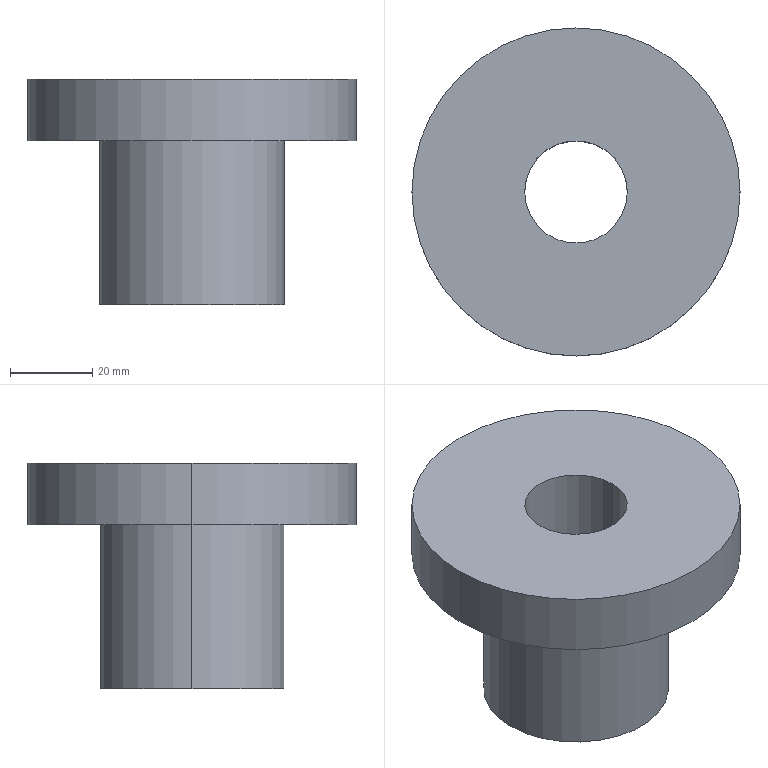Part | SolidWorks | features Cut 1, Extrusion 1, ICE 1 | 1 solid | 9 faces | box 80 x 80 x 55 mm | volume 112017 mm3 | cylinder 6 | plane 3 | commonest cylinder face diameters 25 x2 45 x2 80 x2
STEP:
#1=CARTESIAN_POINT('',(-12.5,0.,55.));
#2=VERTEX_POINT('',#1);
#3=CARTESIAN_POINT('',(12.5,0.,55.));
#4=VERTEX_POINT('',#3);
#5=CARTESIAN_POINT('',(0.,0.,55.));
#6=DIRECTION('',(0.,0.,1.));
#7=DIRECTION('',(1.,0.,0.));
#8=AXIS2_PLACEMENT_3D('',#5,#6,#7);
#9=CIRCLE('',#8,12.5);
#10=EDGE_CURVE('',#2,#4,#9,.T.);
#11=ORIENTED_EDGE('',*,*,#10,.T.);
#12=CARTESIAN_POINT('',(12.5,0.,0.));
#13=VERTEX_POINT('',#12);
#14=CARTESIAN_POINT('',(12.5,0.,97.));
#15=DIRECTION('',(0.,0.,-1.));
#16=VECTOR('',#15,1000.);
#17=LINE('',#14,#16);
#18=EDGE_CURVE('',#4,#13,#17,.T.);
#19=ORIENTED_EDGE('',*,*,#18,.T.);
#20=CARTESIAN_POINT('',(-12.5,0.,0.));
#21=VERTEX_POINT('',#20);
#22=CARTESIAN_POINT('',(0.,0.,0.));
#23=DIRECTION('',(0.,0.,-1.));
#24=DIRECTION('',(-1.,0.,0.));
#25=AXIS2_PLACEMENT_3D('',#22,#23,#24);
#26=CIRCLE('',#25,12.5);
#27=EDGE_CURVE('',#13,#21,#26,.T.);
#28=ORIENTED_EDGE('',*,*,#27,.T.);
#29=CARTESIAN_POINT('',(-12.5,0.,97.));
#30=DIRECTION('',(0.,0.,-1.));
#31=VECTOR('',#30,1000.);
#32=LINE('',#29,#31);
#33=EDGE_CURVE('',#2,#21,#32,.T.);
#34=ORIENTED_EDGE('',*,*,#33,.F.);
#35=EDGE_LOOP('',(#11,#19,#28,#34));
#36=FACE_OUTER_BOUND('',#35,.T.);
#37=CARTESIAN_POINT('',(0.,0.,97.));
#38=DIRECTION('',(0.,0.,-1.));
#39=DIRECTION('',(-1.,0.,0.));
#40=AXIS2_PLACEMENT_3D('',#37,#38,#39);
#41=CYLINDRICAL_SURFACE('',#40,12.5);
#42=ADVANCED_FACE('',(#36),#41,.F.);
#43=CARTESIAN_POINT('',(40.,0.,55.));
#44=VERTEX_POINT('',#43);
#45=CARTESIAN_POINT('',(-40.,0.,55.));
#46=VERTEX_POINT('',#45);
#47=CARTESIAN_POINT('',(0.,0.,55.));
#48=DIRECTION('',(0.,0.,1.));
#49=DIRECTION('',(1.,0.,0.));
#50=AXIS2_PLACEMENT_3D('',#47,#48,#49);
#51=CIRCLE('',#50,40.);
#52=EDGE_CURVE('',#44,#46,#51,.T.);
#53=ORIENTED_EDGE('',*,*,#52,.F.);
#54=CARTESIAN_POINT('',(40.,0.,40.));
#55=VERTEX_POINT('',#54);
#56=CARTESIAN_POINT('',(40.,0.,55.));
#57=DIRECTION('',(0.,0.,-1.));
#58=VECTOR('',#57,1000.);
#59=LINE('',#56,#58);
#60=EDGE_CURVE('',#44,#55,#59,.T.);
#61=ORIENTED_EDGE('',*,*,#60,.T.);
#62=CARTESIAN_POINT('',(-40.,0.,40.));
#63=VERTEX_POINT('',#62);
#64=CARTESIAN_POINT('',(0.,0.,40.));
#65=DIRECTION('',(0.,0.,1.));
#66=DIRECTION('',(1.,0.,0.));
#67=AXIS2_PLACEMENT_3D('',#64,#65,#66);
#68=CIRCLE('',#67,40.);
#69=EDGE_CURVE('',#55,#63,#68,.T.);
#70=ORIENTED_EDGE('',*,*,#69,.T.);
#71=CARTESIAN_POINT('',(-40.,0.,55.));
#72=DIRECTION('',(0.,0.,-1.));
#73=VECTOR('',#72,1000.);
#74=LINE('',#71,#73);
#75=EDGE_CURVE('',#46,#63,#74,.T.);
#76=ORIENTED_EDGE('',*,*,#75,.F.);
#77=EDGE_LOOP('',(#53,#61,#70,#76));
#78=FACE_OUTER_BOUND('',#77,.T.);
#79=CARTESIAN_POINT('',(0.,0.,55.));
#80=DIRECTION('',(0.,0.,-1.));
#81=DIRECTION('',(-1.,0.,0.));
#82=AXIS2_PLACEMENT_3D('',#79,#80,#81);
#83=CYLINDRICAL_SURFACE('',#82,40.);
#84=ADVANCED_FACE('',(#78),#83,.T.);
#85=CARTESIAN_POINT('',(22.5,0.,40.));
#86=VERTEX_POINT('',#85);
#87=CARTESIAN_POINT('',(-22.5,0.,40.));
#88=VERTEX_POINT('',#87);
#89=CARTESIAN_POINT('',(0.,0.,40.));
#90=DIRECTION('',(0.,0.,1.));
#91=DIRECTION('',(1.,0.,0.));
#92=AXIS2_PLACEMENT_3D('',#89,#90,#91);
#93=CIRCLE('',#92,22.5);
#94=EDGE_CURVE('',#86,#88,#93,.T.);
#95=ORIENTED_EDGE('',*,*,#94,.F.);
#96=CARTESIAN_POINT('',(22.5,0.,0.));
#97=VERTEX_POINT('',#96);
#98=CARTESIAN_POINT('',(22.5,0.,40.));
#99=DIRECTION('',(0.,0.,-1.));
#100=VECTOR('',#99,1000.);
#101=LINE('',#98,#100);
#102=EDGE_CURVE('',#86,#97,#101,.T.);
#103=ORIENTED_EDGE('',*,*,#102,.T.);
#104=CARTESIAN_POINT('',(-22.5,0.,0.));
#105=VERTEX_POINT('',#104);
#106=CARTESIAN_POINT('',(0.,0.,0.));
#107=DIRECTION('',(0.,0.,1.));
#108=DIRECTION('',(1.,0.,0.));
#109=AXIS2_PLACEMENT_3D('',#106,#107,#108);
#110=CIRCLE('',#109,22.5);
#111=EDGE_CURVE('',#97,#105,#110,.T.);
#112=ORIENTED_EDGE('',*,*,#111,.T.);
#113=CARTESIAN_POINT('',(-22.5,0.,40.));
#114=DIRECTION('',(0.,0.,-1.));
#115=VECTOR('',#114,1000.);
#116=LINE('',#113,#115);
#117=EDGE_CURVE('',#88,#105,#116,.T.);
#118=ORIENTED_EDGE('',*,*,#117,.F.);
#119=EDGE_LOOP('',(#95,#103,#112,#118));
#120=FACE_OUTER_BOUND('',#119,.T.);
#121=CARTESIAN_POINT('',(0.,0.,40.));
#122=DIRECTION('',(0.,0.,-1.));
#123=DIRECTION('',(-1.,0.,0.));
#124=AXIS2_PLACEMENT_3D('',#121,#122,#123);
#125=CYLINDRICAL_SURFACE('',#124,22.5);
#126=ADVANCED_FACE('',(#120),#125,.T.);
#127=ORIENTED_EDGE('',*,*,#102,.F.);
#128=CARTESIAN_POINT('',(0.,0.,40.));
#129=DIRECTION('',(0.,0.,1.));
#130=DIRECTION('',(1.,0.,0.));
#131=AXIS2_PLACEMENT_3D('',#128,#129,#130);
#132=CIRCLE('',#131,22.5);
#133=EDGE_CURVE('',#88,#86,#132,.T.);
#134=ORIENTED_EDGE('',*,*,#133,.F.);
#135=ORIENTED_EDGE('',*,*,#117,.T.);
#136=CARTESIAN_POINT('',(0.,0.,0.));
#137=DIRECTION('',(0.,0.,1.));
#138=DIRECTION('',(1.,0.,0.));
#139=AXIS2_PLACEMENT_3D('',#136,#137,#138);
#140=CIRCLE('',#139,22.5);
#141=EDGE_CURVE('',#105,#97,#140,.T.);
#142=ORIENTED_EDGE('',*,*,#141,.T.);
#143=EDGE_LOOP('',(#127,#134,#135,#142));
#144=FACE_OUTER_BOUND('',#143,.T.);
#145=CARTESIAN_POINT('',(0.,0.,40.));
#146=DIRECTION('',(0.,0.,-1.));
#147=DIRECTION('',(-1.,0.,0.));
#148=AXIS2_PLACEMENT_3D('',#145,#146,#147);
#149=CYLINDRICAL_SURFACE('',#148,22.5);
#150=ADVANCED_FACE('',(#144),#149,.T.);
#151=CARTESIAN_POINT('',(0.,0.,0.));
#152=DIRECTION('',(0.,0.,-1.));
#153=DIRECTION('',(-1.,0.,0.));
#154=AXIS2_PLACEMENT_3D('',#151,#152,#153);
#155=CIRCLE('',#154,12.5);
#156=EDGE_CURVE('',#21,#13,#155,.T.);
#157=ORIENTED_EDGE('',*,*,#156,.F.);
#158=ORIENTED_EDGE('',*,*,#27,.F.);
#159=EDGE_LOOP('',(#157,#158));
#160=FACE_BOUND('',#159,.T.);
#161=ORIENTED_EDGE('',*,*,#141,.F.);
#162=ORIENTED_EDGE('',*,*,#111,.F.);
#163=EDGE_LOOP('',(#161,#162));
#164=FACE_OUTER_BOUND('',#163,.T.);
#165=CARTESIAN_POINT('',(0.,0.,0.));
#166=DIRECTION('',(0.,0.,1.));
#167=DIRECTION('',(1.,0.,0.));
#168=AXIS2_PLACEMENT_3D('',#165,#166,#167);
#169=PLANE('',#168);
#170=ADVANCED_FACE('',(#160,#164),#169,.F.);
#171=ORIENTED_EDGE('',*,*,#60,.F.);
#172=CARTESIAN_POINT('',(0.,0.,55.));
#173=DIRECTION('',(0.,0.,1.));
#174=DIRECTION('',(1.,0.,0.));
#175=AXIS2_PLACEMENT_3D('',#172,#173,#174);
#176=CIRCLE('',#175,40.);
#177=EDGE_CURVE('',#46,#44,#176,.T.);
#178=ORIENTED_EDGE('',*,*,#177,.F.);
#179=ORIENTED_EDGE('',*,*,#75,.T.);
#180=CARTESIAN_POINT('',(0.,0.,40.));
#181=DIRECTION('',(0.,0.,1.));
#182=DIRECTION('',(1.,0.,0.));
#183=AXIS2_PLACEMENT_3D('',#180,#181,#182);
#184=CIRCLE('',#183,40.);
#185=EDGE_CURVE('',#63,#55,#184,.T.);
#186=ORIENTED_EDGE('',*,*,#185,.T.);
#187=EDGE_LOOP('',(#171,#178,#179,#186));
#188=FACE_OUTER_BOUND('',#187,.T.);
#189=CARTESIAN_POINT('',(0.,0.,55.));
#190=DIRECTION('',(0.,0.,-1.));
#191=DIRECTION('',(-1.,0.,0.));
#192=AXIS2_PLACEMENT_3D('',#189,#190,#191);
#193=CYLINDRICAL_SURFACE('',#192,40.);
#194=ADVANCED_FACE('',(#188),#193,.T.);
#195=ORIENTED_EDGE('',*,*,#10,.F.);
#196=CARTESIAN_POINT('',(0.,0.,55.));
#197=DIRECTION('',(0.,0.,1.));
#198=DIRECTION('',(1.,0.,0.));
#199=AXIS2_PLACEMENT_3D('',#196,#197,#198);
#200=CIRCLE('',#199,12.5);
#201=EDGE_CURVE('',#4,#2,#200,.T.);
#202=ORIENTED_EDGE('',*,*,#201,.F.);
#203=EDGE_LOOP('',(#195,#202));
#204=FACE_BOUND('',#203,.T.);
#205=ORIENTED_EDGE('',*,*,#177,.T.);
#206=ORIENTED_EDGE('',*,*,#52,.T.);
#207=EDGE_LOOP('',(#205,#206));
#208=FACE_OUTER_BOUND('',#207,.T.);
#209=CARTESIAN_POINT('',(0.,0.,55.));
#210=DIRECTION('',(0.,0.,1.));
#211=DIRECTION('',(1.,0.,0.));
#212=AXIS2_PLACEMENT_3D('',#209,#210,#211);
#213=PLANE('',#212);
#214=ADVANCED_FACE('',(#204,#208),#213,.T.);
#215=ORIENTED_EDGE('',*,*,#133,.T.);
#216=ORIENTED_EDGE('',*,*,#94,.T.);
#217=EDGE_LOOP('',(#215,#216));
#218=FACE_BOUND('',#217,.T.);
#219=ORIENTED_EDGE('',*,*,#185,.F.);
#220=ORIENTED_EDGE('',*,*,#69,.F.);
#221=EDGE_LOOP('',(#219,#220));
#222=FACE_OUTER_BOUND('',#221,.T.);
#223=CARTESIAN_POINT('',(0.,0.,40.));
#224=DIRECTION('',(0.,0.,1.));
#225=DIRECTION('',(1.,0.,0.));
#226=AXIS2_PLACEMENT_3D('',#223,#224,#225);
#227=PLANE('',#226);
#228=ADVANCED_FACE('',(#218,#222),#227,.F.);
#229=ORIENTED_EDGE('',*,*,#18,.F.);
#230=ORIENTED_EDGE('',*,*,#201,.T.);
#231=ORIENTED_EDGE('',*,*,#33,.T.);
#232=ORIENTED_EDGE('',*,*,#156,.T.);
#233=EDGE_LOOP('',(#229,#230,#231,#232));
#234=FACE_OUTER_BOUND('',#233,.T.);
#235=CARTESIAN_POINT('',(0.,0.,97.));
#236=DIRECTION('',(0.,0.,-1.));
#237=DIRECTION('',(-1.,0.,0.));
#238=AXIS2_PLACEMENT_3D('',#235,#236,#237);
#239=CYLINDRICAL_SURFACE('',#238,12.5);
#240=ADVANCED_FACE('',(#234),#239,.F.);
#241=CLOSED_SHELL('',(#42,#84,#126,#150,#170,#194,#214,#228,#240));
#242=MANIFOLD_SOLID_BREP('',#241);
#243=CARTESIAN_POINT('',(0.,0.,0.));
#244=DIRECTION('',(0.,0.,1.));
#245=DIRECTION('',(1.,0.,0.));
#246=AXIS2_PLACEMENT_3D('',#243,#244,#245);
#247=(LENGTH_UNIT()NAMED_UNIT(*)SI_UNIT(.MILLI.,.METRE.));
#248=UNCERTAINTY_MEASURE_WITH_UNIT(LENGTH_MEASURE(0.00001),#247,'','');
#249=(NAMED_UNIT(*)PLANE_ANGLE_UNIT()SI_UNIT($,.RADIAN.));
#250=(NAMED_UNIT(*)SI_UNIT($,.STERADIAN.)SOLID_ANGLE_UNIT());
#251=(GEOMETRIC_REPRESENTATION_CONTEXT(3)GLOBAL_UNCERTAINTY_ASSIGNED_CONTEXT((#248))GLOBAL_UNIT_ASSIGNED_CONTEXT((#247,#249,#250))REPRESENTATION_CONTEXT('',''));
#252=ADVANCED_BREP_SHAPE_REPRESENTATION('',(#242,#246),#251);